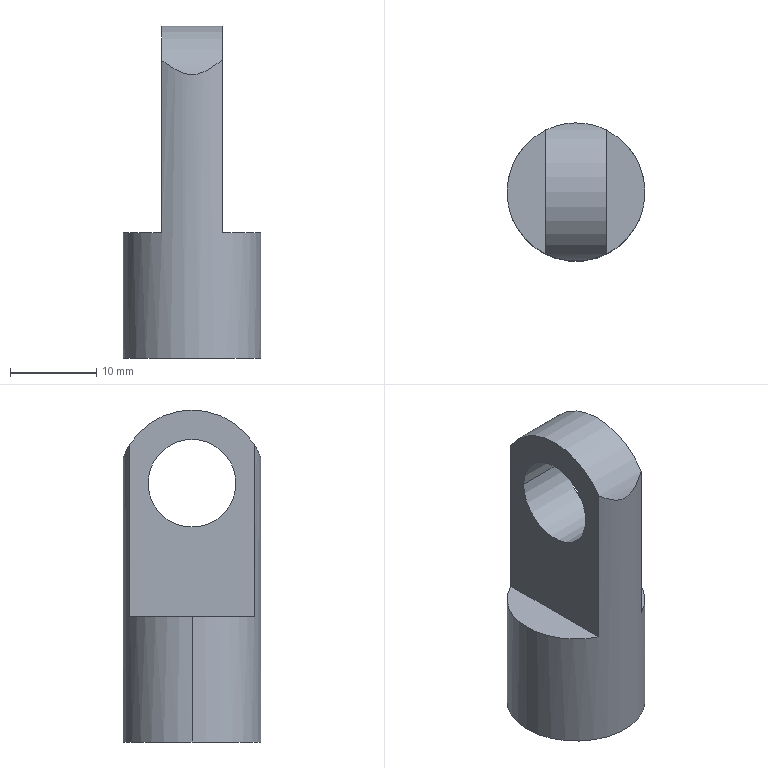Part | SolidWorks | features ICE 3, Extrusion 1, HoleWzd 1 | 1 solid | 14 faces | box 16 x 16 x 38.5 mm | volume 4330 mm3 | cylinder 7 | plane 5 | cone 2 | commonest cylinder face diameters 6.8 x2 10.2 x2 16 x2 17 x1
STEP:
#1=CARTESIAN_POINT('',(3.4,0.,12.));
#2=VERTEX_POINT('',#1);
#3=CARTESIAN_POINT('',(-3.4,0.,12.));
#4=VERTEX_POINT('',#3);
#5=CARTESIAN_POINT('',(0.,0.,12.));
#6=DIRECTION('',(0.,0.,-1.));
#7=DIRECTION('',(-1.,0.,0.));
#8=AXIS2_PLACEMENT_3D('',#5,#6,#7);
#9=CIRCLE('',#8,3.4);
#10=EDGE_CURVE('',#2,#4,#9,.T.);
#11=ORIENTED_EDGE('',*,*,#10,.F.);
#12=CARTESIAN_POINT('',(3.4,0.,0.));
#13=VERTEX_POINT('',#12);
#14=CARTESIAN_POINT('',(3.4,0.,0.));
#15=DIRECTION('',(0.,0.,-1.));
#16=VECTOR('',#15,1000.);
#17=LINE('',#14,#16);
#18=EDGE_CURVE('',#2,#13,#17,.T.);
#19=ORIENTED_EDGE('',*,*,#18,.T.);
#20=CARTESIAN_POINT('',(-3.4,0.,0.));
#21=VERTEX_POINT('',#20);
#22=CARTESIAN_POINT('',(0.,0.,0.));
#23=DIRECTION('',(0.,0.,-1.));
#24=DIRECTION('',(-1.,0.,0.));
#25=AXIS2_PLACEMENT_3D('',#22,#23,#24);
#26=CIRCLE('',#25,3.4);
#27=EDGE_CURVE('',#13,#21,#26,.T.);
#28=ORIENTED_EDGE('',*,*,#27,.T.);
#29=CARTESIAN_POINT('',(-3.4,0.,0.));
#30=DIRECTION('',(0.,0.,-1.));
#31=VECTOR('',#30,1000.);
#32=LINE('',#29,#31);
#33=EDGE_CURVE('',#4,#21,#32,.T.);
#34=ORIENTED_EDGE('',*,*,#33,.F.);
#35=EDGE_LOOP('',(#11,#19,#28,#34));
#36=FACE_OUTER_BOUND('',#35,.T.);
#37=CARTESIAN_POINT('',(0.,0.,0.));
#38=DIRECTION('',(0.,0.,-1.));
#39=DIRECTION('',(-1.,0.,0.));
#40=AXIS2_PLACEMENT_3D('',#37,#38,#39);
#41=CYLINDRICAL_SURFACE('',#40,3.4);
#42=ADVANCED_FACE('',(#36),#41,.F.);
#43=CARTESIAN_POINT('',(0.,0.,14.043));
#44=VERTEX_POINT('',#43);
#45=CARTESIAN_POINT('',(-3.4,0.,12.));
#46=DIRECTION('',(-0.8572,0.,-0.515));
#47=VECTOR('',#46,1000.);
#48=LINE('',#45,#47);
#49=EDGE_CURVE('',#44,#4,#48,.T.);
#50=ORIENTED_EDGE('',*,*,#49,.F.);
#51=CARTESIAN_POINT('',(3.4,0.,12.));
#52=DIRECTION('',(0.8572,0.,-0.515));
#53=VECTOR('',#52,1000.);
#54=LINE('',#51,#53);
#55=EDGE_CURVE('',#44,#2,#54,.T.);
#56=ORIENTED_EDGE('',*,*,#55,.T.);
#57=ORIENTED_EDGE('',*,*,#10,.T.);
#58=EDGE_LOOP('',(#50,#56,#57));
#59=FACE_OUTER_BOUND('',#58,.T.);
#60=CARTESIAN_POINT('',(0.,0.,12.));
#61=DIRECTION('',(0.,0.,-1.));
#62=DIRECTION('',(-1.,0.,0.));
#63=AXIS2_PLACEMENT_3D('',#60,#61,#62);
#64=CONICAL_SURFACE('',#63,3.4,1.03);
#65=ADVANCED_FACE('',(#59),#64,.F.);
#66=CARTESIAN_POINT('',(-3.5,-5.1,30.));
#67=VERTEX_POINT('',#66);
#68=CARTESIAN_POINT('',(-3.5,5.1,30.));
#69=VERTEX_POINT('',#68);
#70=CARTESIAN_POINT('',(-3.5,0.,30.));
#71=DIRECTION('',(1.,0.,0.));
#72=DIRECTION('',(0.,0.,-1.));
#73=AXIS2_PLACEMENT_3D('',#70,#71,#72);
#74=CIRCLE('',#73,5.1);
#75=EDGE_CURVE('',#67,#69,#74,.T.);
#76=ORIENTED_EDGE('',*,*,#75,.F.);
#77=CARTESIAN_POINT('',(3.5,-5.1,30.));
#78=VERTEX_POINT('',#77);
#79=CARTESIAN_POINT('',(-20.5,-5.1,30.));
#80=DIRECTION('',(1.,0.,0.));
#81=VECTOR('',#80,1000.);
#82=LINE('',#79,#81);
#83=EDGE_CURVE('',#67,#78,#82,.T.);
#84=ORIENTED_EDGE('',*,*,#83,.T.);
#85=CARTESIAN_POINT('',(3.5,5.1,30.));
#86=VERTEX_POINT('',#85);
#87=CARTESIAN_POINT('',(3.5,0.,30.));
#88=DIRECTION('',(1.,0.,0.));
#89=DIRECTION('',(0.,1.,0.));
#90=AXIS2_PLACEMENT_3D('',#87,#88,#89);
#91=CIRCLE('',#90,5.1);
#92=EDGE_CURVE('',#78,#86,#91,.T.);
#93=ORIENTED_EDGE('',*,*,#92,.T.);
#94=CARTESIAN_POINT('',(-20.5,5.1,30.));
#95=DIRECTION('',(1.,0.,0.));
#96=VECTOR('',#95,1000.);
#97=LINE('',#94,#96);
#98=EDGE_CURVE('',#69,#86,#97,.T.);
#99=ORIENTED_EDGE('',*,*,#98,.F.);
#100=EDGE_LOOP('',(#76,#84,#93,#99));
#101=FACE_OUTER_BOUND('',#100,.T.);
#102=CARTESIAN_POINT('',(-20.5,0.,30.));
#103=DIRECTION('',(1.,0.,0.));
#104=DIRECTION('',(0.,1.,0.));
#105=AXIS2_PLACEMENT_3D('',#102,#103,#104);
#106=CYLINDRICAL_SURFACE('',#105,5.1);
#107=ADVANCED_FACE('',(#101),#106,.F.);
#108=CARTESIAN_POINT('',(8.,0.,14.5));
#109=VERTEX_POINT('',#108);
#110=CARTESIAN_POINT('',(3.5,7.194,14.5));
#111=VERTEX_POINT('',#110);
#112=CARTESIAN_POINT('',(0.,0.,14.5));
#113=DIRECTION('',(0.,0.,1.));
#114=DIRECTION('',(1.,0.,0.));
#115=AXIS2_PLACEMENT_3D('',#112,#113,#114);
#116=CIRCLE('',#115,8.);
#117=EDGE_CURVE('',#109,#111,#116,.T.);
#118=ORIENTED_EDGE('',*,*,#117,.F.);
#119=CARTESIAN_POINT('',(8.,0.,0.));
#120=VERTEX_POINT('',#119);
#121=CARTESIAN_POINT('',(8.,0.,38.5));
#122=DIRECTION('',(0.,0.,-1.));
#123=VECTOR('',#122,1000.);
#124=LINE('',#121,#123);
#125=EDGE_CURVE('',#109,#120,#124,.T.);
#126=ORIENTED_EDGE('',*,*,#125,.T.);
#127=CARTESIAN_POINT('',(-8.,0.,0.));
#128=VERTEX_POINT('',#127);
#129=CARTESIAN_POINT('',(0.,0.,0.));
#130=DIRECTION('',(0.,0.,1.));
#131=DIRECTION('',(1.,0.,0.));
#132=AXIS2_PLACEMENT_3D('',#129,#130,#131);
#133=CIRCLE('',#132,8.);
#134=EDGE_CURVE('',#120,#128,#133,.T.);
#135=ORIENTED_EDGE('',*,*,#134,.T.);
#136=CARTESIAN_POINT('',(-8.,0.,14.5));
#137=VERTEX_POINT('',#136);
#138=CARTESIAN_POINT('',(-8.,0.,38.5));
#139=DIRECTION('',(0.,0.,-1.));
#140=VECTOR('',#139,1000.);
#141=LINE('',#138,#140);
#142=EDGE_CURVE('',#137,#128,#141,.T.);
#143=ORIENTED_EDGE('',*,*,#142,.F.);
#144=CARTESIAN_POINT('',(-3.5,7.194,14.5));
#145=VERTEX_POINT('',#144);
#146=CARTESIAN_POINT('',(0.,0.,14.5));
#147=DIRECTION('',(0.,0.,1.));
#148=DIRECTION('',(1.,0.,0.));
#149=AXIS2_PLACEMENT_3D('',#146,#147,#148);
#150=CIRCLE('',#149,8.);
#151=EDGE_CURVE('',#145,#137,#150,.T.);
#152=ORIENTED_EDGE('',*,*,#151,.F.);
#153=CARTESIAN_POINT('',(-3.5,7.194,34.528));
#154=VERTEX_POINT('',#153);
#155=CARTESIAN_POINT('',(-3.5,7.194,38.5));
#156=DIRECTION('',(0.,0.,1.));
#157=VECTOR('',#156,1000.);
#158=LINE('',#155,#157);
#159=EDGE_CURVE('',#145,#154,#158,.T.);
#160=ORIENTED_EDGE('',*,*,#159,.T.);
#161=CARTESIAN_POINT('',(3.5,7.194,34.528));
#162=VERTEX_POINT('',#161);
#163=CARTESIAN_POINT('',(-3.5,7.194,34.528));
#164=CARTESIAN_POINT('',(-3.254,7.314,34.337));
#165=CARTESIAN_POINT('',(-2.999,7.422,34.148));
#166=CARTESIAN_POINT('',(-2.468,7.615,33.782));
#167=CARTESIAN_POINT('',(-2.191,7.7,33.605));
#168=CARTESIAN_POINT('',(-1.758,7.806,33.365));
#169=CARTESIAN_POINT('',(-1.61,7.838,33.29));
#170=CARTESIAN_POINT('',(-1.307,7.894,33.153));
#171=CARTESIAN_POINT('',(-1.15,7.919,33.09));
#172=CARTESIAN_POINT('',(-0.8316,7.958,32.986));
#173=CARTESIAN_POINT('',(-0.6695,7.974,32.945));
#174=CARTESIAN_POINT('',(-0.3382,7.995,32.888));
#175=CARTESIAN_POINT('',(-0.167,8.,32.872));
#176=CARTESIAN_POINT('',(0.1699,8.,32.872));
#177=CARTESIAN_POINT('',(0.3366,7.995,32.887));
#178=CARTESIAN_POINT('',(0.6668,7.974,32.944));
#179=CARTESIAN_POINT('',(0.8317,7.958,32.986));
#180=CARTESIAN_POINT('',(1.31,7.899,33.143));
#181=CARTESIAN_POINT('',(1.609,7.842,33.284));
#182=CARTESIAN_POINT('',(2.186,7.701,33.602));
#183=CARTESIAN_POINT('',(2.463,7.617,33.779));
#184=CARTESIAN_POINT('',(2.994,7.424,34.145));
#185=CARTESIAN_POINT('',(3.251,7.315,34.335));
#186=CARTESIAN_POINT('',(3.5,7.194,34.528));
#187=B_SPLINE_CURVE_WITH_KNOTS('',3,(#163,#164,#165,#166,#167,#168,#169,#170,#171,#172,#173,#174,#175,#176,#177,#178,#179,#180,#181,#182,#183,#184,#185,#186),.UNSPECIFIED.,.F.,.F.,(4,2,2,2,2,2,2,2,2,2,2,4),(0.009914,0.01092,0.01192,0.01242,0.01292,0.01343,0.01393,0.01443,0.01493,0.01593,0.01694,0.01794),.UNSPECIFIED.);
#188=EDGE_CURVE('',#154,#162,#187,.T.);
#189=ORIENTED_EDGE('',*,*,#188,.T.);
#190=CARTESIAN_POINT('',(3.5,7.194,38.5));
#191=DIRECTION('',(0.,0.,-1.));
#192=VECTOR('',#191,1000.);
#193=LINE('',#190,#192);
#194=EDGE_CURVE('',#162,#111,#193,.T.);
#195=ORIENTED_EDGE('',*,*,#194,.T.);
#196=EDGE_LOOP('',(#118,#126,#135,#143,#152,#160,#189,#195));
#197=FACE_OUTER_BOUND('',#196,.T.);
#198=CARTESIAN_POINT('',(0.,0.,38.5));
#199=DIRECTION('',(0.,0.,-1.));
#200=DIRECTION('',(-1.,0.,0.));
#201=AXIS2_PLACEMENT_3D('',#198,#199,#200);
#202=CYLINDRICAL_SURFACE('',#201,8.);
#203=ADVANCED_FACE('',(#197),#202,.T.);
#204=CARTESIAN_POINT('',(-3.5,0.,30.));
#205=DIRECTION('',(1.,0.,0.));
#206=DIRECTION('',(0.,0.,-1.));
#207=AXIS2_PLACEMENT_3D('',#204,#205,#206);
#208=CIRCLE('',#207,5.1);
#209=EDGE_CURVE('',#69,#67,#208,.T.);
#210=ORIENTED_EDGE('',*,*,#209,.T.);
#211=ORIENTED_EDGE('',*,*,#75,.T.);
#212=EDGE_LOOP('',(#210,#211));
#213=FACE_BOUND('',#212,.T.);
#214=CARTESIAN_POINT('',(-3.5,-7.194,34.528));
#215=VERTEX_POINT('',#214);
#216=CARTESIAN_POINT('',(-3.5,-7.194,14.5));
#217=VERTEX_POINT('',#216);
#218=CARTESIAN_POINT('',(-3.5,-7.194,38.5));
#219=DIRECTION('',(0.,0.,-1.));
#220=VECTOR('',#219,1000.);
#221=LINE('',#218,#220);
#222=EDGE_CURVE('',#215,#217,#221,.T.);
#223=ORIENTED_EDGE('',*,*,#222,.F.);
#224=CARTESIAN_POINT('',(-3.5,0.,30.));
#225=DIRECTION('',(-1.,0.,0.));
#226=DIRECTION('',(0.,0.,-1.));
#227=AXIS2_PLACEMENT_3D('',#224,#225,#226);
#228=CIRCLE('',#227,8.5);
#229=EDGE_CURVE('',#215,#154,#228,.T.);
#230=ORIENTED_EDGE('',*,*,#229,.T.);
#231=ORIENTED_EDGE('',*,*,#159,.F.);
#232=CARTESIAN_POINT('',(-3.5,8.,14.5));
#233=DIRECTION('',(0.,1.,0.));
#234=VECTOR('',#233,1000.);
#235=LINE('',#232,#234);
#236=EDGE_CURVE('',#217,#145,#235,.T.);
#237=ORIENTED_EDGE('',*,*,#236,.F.);
#238=EDGE_LOOP('',(#223,#230,#231,#237));
#239=FACE_OUTER_BOUND('',#238,.T.);
#240=CARTESIAN_POINT('',(-3.5,8.,14.5));
#241=DIRECTION('',(1.,0.,0.));
#242=DIRECTION('',(0.,0.,-1.));
#243=AXIS2_PLACEMENT_3D('',#240,#241,#242);
#244=PLANE('',#243);
#245=ADVANCED_FACE('',(#213,#239),#244,.F.);
#246=CARTESIAN_POINT('',(3.5,0.,30.));
#247=DIRECTION('',(1.,0.,0.));
#248=DIRECTION('',(0.,1.,0.));
#249=AXIS2_PLACEMENT_3D('',#246,#247,#248);
#250=CIRCLE('',#249,5.1);
#251=EDGE_CURVE('',#86,#78,#250,.T.);
#252=ORIENTED_EDGE('',*,*,#251,.F.);
#253=ORIENTED_EDGE('',*,*,#92,.F.);
#254=EDGE_LOOP('',(#252,#253));
#255=FACE_BOUND('',#254,.T.);
#256=ORIENTED_EDGE('',*,*,#194,.F.);
#257=CARTESIAN_POINT('',(3.5,-7.194,34.528));
#258=VERTEX_POINT('',#257);
#259=CARTESIAN_POINT('',(3.5,0.,30.));
#260=DIRECTION('',(1.,0.,0.));
#261=DIRECTION('',(0.,-1.,0.));
#262=AXIS2_PLACEMENT_3D('',#259,#260,#261);
#263=CIRCLE('',#262,8.5);
#264=EDGE_CURVE('',#162,#258,#263,.T.);
#265=ORIENTED_EDGE('',*,*,#264,.T.);
#266=CARTESIAN_POINT('',(3.5,-7.194,14.5));
#267=VERTEX_POINT('',#266);
#268=CARTESIAN_POINT('',(3.5,-7.194,38.5));
#269=DIRECTION('',(0.,0.,1.));
#270=VECTOR('',#269,1000.);
#271=LINE('',#268,#270);
#272=EDGE_CURVE('',#267,#258,#271,.T.);
#273=ORIENTED_EDGE('',*,*,#272,.F.);
#274=CARTESIAN_POINT('',(3.5,8.,14.5));
#275=DIRECTION('',(0.,-1.,0.));
#276=VECTOR('',#275,1000.);
#277=LINE('',#274,#276);
#278=EDGE_CURVE('',#111,#267,#277,.T.);
#279=ORIENTED_EDGE('',*,*,#278,.F.);
#280=EDGE_LOOP('',(#256,#265,#273,#279));
#281=FACE_OUTER_BOUND('',#280,.T.);
#282=CARTESIAN_POINT('',(3.5,8.,14.5));
#283=DIRECTION('',(-1.,0.,0.));
#284=DIRECTION('',(0.,-1.,0.));
#285=AXIS2_PLACEMENT_3D('',#282,#283,#284);
#286=PLANE('',#285);
#287=ADVANCED_FACE('',(#255,#281),#286,.F.);
#288=ORIENTED_EDGE('',*,*,#125,.F.);
#289=CARTESIAN_POINT('',(0.,0.,14.5));
#290=DIRECTION('',(0.,0.,1.));
#291=DIRECTION('',(1.,0.,0.));
#292=AXIS2_PLACEMENT_3D('',#289,#290,#291);
#293=CIRCLE('',#292,8.);
#294=EDGE_CURVE('',#267,#109,#293,.T.);
#295=ORIENTED_EDGE('',*,*,#294,.F.);
#296=ORIENTED_EDGE('',*,*,#272,.T.);
#297=CARTESIAN_POINT('',(3.5,-7.194,34.528));
#298=CARTESIAN_POINT('',(3.25,-7.315,34.335));
#299=CARTESIAN_POINT('',(2.994,-7.424,34.145));
#300=CARTESIAN_POINT('',(2.463,-7.617,33.779));
#301=CARTESIAN_POINT('',(2.186,-7.701,33.602));
#302=CARTESIAN_POINT('',(1.609,-7.842,33.283));
#303=CARTESIAN_POINT('',(1.309,-7.899,33.142));
#304=CARTESIAN_POINT('',(0.8311,-7.958,32.986));
#305=CARTESIAN_POINT('',(0.666,-7.974,32.944));
#306=CARTESIAN_POINT('',(0.3347,-7.995,32.887));
#307=CARTESIAN_POINT('',(0.1674,-8.,32.872));
#308=CARTESIAN_POINT('',(-0.1706,-8.,32.872));
#309=CARTESIAN_POINT('',(-0.3414,-7.994,32.888));
#310=CARTESIAN_POINT('',(-0.6727,-7.973,32.945));
#311=CARTESIAN_POINT('',(-0.8351,-7.958,32.987));
#312=CARTESIAN_POINT('',(-1.155,-7.918,33.092));
#313=CARTESIAN_POINT('',(-1.311,-7.893,33.155));
#314=CARTESIAN_POINT('',(-1.613,-7.837,33.292));
#315=CARTESIAN_POINT('',(-1.76,-7.805,33.367));
#316=CARTESIAN_POINT('',(-2.191,-7.7,33.605));
#317=CARTESIAN_POINT('',(-2.466,-7.616,33.781));
#318=CARTESIAN_POINT('',(-2.999,-7.422,34.148));
#319=CARTESIAN_POINT('',(-3.253,-7.314,34.337));
#320=CARTESIAN_POINT('',(-3.5,-7.194,34.528));
#321=B_SPLINE_CURVE_WITH_KNOTS('',3,(#297,#298,#299,#300,#301,#302,#303,#304,#305,#306,#307,#308,#309,#310,#311,#312,#313,#314,#315,#316,#317,#318,#319,#320),.UNSPECIFIED.,.F.,.F.,(4,2,2,2,2,2,2,2,2,2,2,4),(0.,0.00101,0.00202,0.003031,0.003536,0.004041,0.004546,0.005051,0.005556,0.006061,0.007072,0.008082),.UNSPECIFIED.);
#322=EDGE_CURVE('',#258,#215,#321,.T.);
#323=ORIENTED_EDGE('',*,*,#322,.T.);
#324=ORIENTED_EDGE('',*,*,#222,.T.);
#325=CARTESIAN_POINT('',(0.,0.,14.5));
#326=DIRECTION('',(0.,0.,1.));
#327=DIRECTION('',(1.,0.,0.));
#328=AXIS2_PLACEMENT_3D('',#325,#326,#327);
#329=CIRCLE('',#328,8.);
#330=EDGE_CURVE('',#137,#217,#329,.T.);
#331=ORIENTED_EDGE('',*,*,#330,.F.);
#332=ORIENTED_EDGE('',*,*,#142,.T.);
#333=CARTESIAN_POINT('',(0.,0.,0.));
#334=DIRECTION('',(0.,0.,1.));
#335=DIRECTION('',(1.,0.,0.));
#336=AXIS2_PLACEMENT_3D('',#333,#334,#335);
#337=CIRCLE('',#336,8.);
#338=EDGE_CURVE('',#128,#120,#337,.T.);
#339=ORIENTED_EDGE('',*,*,#338,.T.);
#340=EDGE_LOOP('',(#288,#295,#296,#323,#324,#331,#332,#339));
#341=FACE_OUTER_BOUND('',#340,.T.);
#342=CARTESIAN_POINT('',(0.,0.,38.5));
#343=DIRECTION('',(0.,0.,-1.));
#344=DIRECTION('',(-1.,0.,0.));
#345=AXIS2_PLACEMENT_3D('',#342,#343,#344);
#346=CYLINDRICAL_SURFACE('',#345,8.);
#347=ADVANCED_FACE('',(#341),#346,.T.);
#348=CARTESIAN_POINT('',(0.,0.,0.));
#349=DIRECTION('',(0.,0.,-1.));
#350=DIRECTION('',(-1.,0.,0.));
#351=AXIS2_PLACEMENT_3D('',#348,#349,#350);
#352=CIRCLE('',#351,3.4);
#353=EDGE_CURVE('',#21,#13,#352,.T.);
#354=ORIENTED_EDGE('',*,*,#353,.F.);
#355=ORIENTED_EDGE('',*,*,#27,.F.);
#356=EDGE_LOOP('',(#354,#355));
#357=FACE_BOUND('',#356,.T.);
#358=ORIENTED_EDGE('',*,*,#338,.F.);
#359=ORIENTED_EDGE('',*,*,#134,.F.);
#360=EDGE_LOOP('',(#358,#359));
#361=FACE_OUTER_BOUND('',#360,.T.);
#362=CARTESIAN_POINT('',(0.,0.,0.));
#363=DIRECTION('',(0.,0.,1.));
#364=DIRECTION('',(1.,0.,0.));
#365=AXIS2_PLACEMENT_3D('',#362,#363,#364);
#366=PLANE('',#365);
#367=ADVANCED_FACE('',(#357,#361),#366,.F.);
#368=ORIENTED_EDGE('',*,*,#151,.T.);
#369=ORIENTED_EDGE('',*,*,#330,.T.);
#370=ORIENTED_EDGE('',*,*,#236,.T.);
#371=EDGE_LOOP('',(#368,#369,#370));
#372=FACE_OUTER_BOUND('',#371,.T.);
#373=CARTESIAN_POINT('',(0.,0.,14.5));
#374=DIRECTION('',(0.,0.,1.));
#375=DIRECTION('',(1.,0.,0.));
#376=AXIS2_PLACEMENT_3D('',#373,#374,#375);
#377=PLANE('',#376);
#378=ADVANCED_FACE('',(#372),#377,.T.);
#379=ORIENTED_EDGE('',*,*,#294,.T.);
#380=ORIENTED_EDGE('',*,*,#117,.T.);
#381=ORIENTED_EDGE('',*,*,#278,.T.);
#382=EDGE_LOOP('',(#379,#380,#381));
#383=FACE_OUTER_BOUND('',#382,.T.);
#384=CARTESIAN_POINT('',(0.,0.,14.5));
#385=DIRECTION('',(0.,0.,1.));
#386=DIRECTION('',(1.,0.,0.));
#387=AXIS2_PLACEMENT_3D('',#384,#385,#386);
#388=PLANE('',#387);
#389=ADVANCED_FACE('',(#383),#388,.T.);
#390=ORIENTED_EDGE('',*,*,#83,.F.);
#391=ORIENTED_EDGE('',*,*,#209,.F.);
#392=ORIENTED_EDGE('',*,*,#98,.T.);
#393=ORIENTED_EDGE('',*,*,#251,.T.);
#394=EDGE_LOOP('',(#390,#391,#392,#393));
#395=FACE_OUTER_BOUND('',#394,.T.);
#396=CARTESIAN_POINT('',(-20.5,0.,30.));
#397=DIRECTION('',(1.,0.,0.));
#398=DIRECTION('',(0.,1.,0.));
#399=AXIS2_PLACEMENT_3D('',#396,#397,#398);
#400=CYLINDRICAL_SURFACE('',#399,5.1);
#401=ADVANCED_FACE('',(#395),#400,.F.);
#402=ORIENTED_EDGE('',*,*,#264,.F.);
#403=ORIENTED_EDGE('',*,*,#188,.F.);
#404=ORIENTED_EDGE('',*,*,#229,.F.);
#405=ORIENTED_EDGE('',*,*,#322,.F.);
#406=EDGE_LOOP('',(#402,#403,#404,#405));
#407=FACE_OUTER_BOUND('',#406,.T.);
#408=CARTESIAN_POINT('',(-8.,0.,30.));
#409=DIRECTION('',(1.,0.,0.));
#410=DIRECTION('',(0.,1.,0.));
#411=AXIS2_PLACEMENT_3D('',#408,#409,#410);
#412=CYLINDRICAL_SURFACE('',#411,8.5);
#413=ADVANCED_FACE('',(#407),#412,.T.);
#414=ORIENTED_EDGE('',*,*,#55,.F.);
#415=ORIENTED_EDGE('',*,*,#49,.T.);
#416=CARTESIAN_POINT('',(0.,0.,12.));
#417=DIRECTION('',(0.,0.,-1.));
#418=DIRECTION('',(-1.,0.,0.));
#419=AXIS2_PLACEMENT_3D('',#416,#417,#418);
#420=CIRCLE('',#419,3.4);
#421=EDGE_CURVE('',#4,#2,#420,.T.);
#422=ORIENTED_EDGE('',*,*,#421,.T.);
#423=EDGE_LOOP('',(#414,#415,#422));
#424=FACE_OUTER_BOUND('',#423,.T.);
#425=CARTESIAN_POINT('',(0.,0.,12.));
#426=DIRECTION('',(0.,0.,-1.));
#427=DIRECTION('',(-1.,0.,0.));
#428=AXIS2_PLACEMENT_3D('',#425,#426,#427);
#429=CONICAL_SURFACE('',#428,3.4,1.03);
#430=ADVANCED_FACE('',(#424),#429,.F.);
#431=ORIENTED_EDGE('',*,*,#18,.F.);
#432=ORIENTED_EDGE('',*,*,#421,.F.);
#433=ORIENTED_EDGE('',*,*,#33,.T.);
#434=ORIENTED_EDGE('',*,*,#353,.T.);
#435=EDGE_LOOP('',(#431,#432,#433,#434));
#436=FACE_OUTER_BOUND('',#435,.T.);
#437=CARTESIAN_POINT('',(0.,0.,0.));
#438=DIRECTION('',(0.,0.,-1.));
#439=DIRECTION('',(-1.,0.,0.));
#440=AXIS2_PLACEMENT_3D('',#437,#438,#439);
#441=CYLINDRICAL_SURFACE('',#440,3.4);
#442=ADVANCED_FACE('',(#436),#441,.F.);
#443=CLOSED_SHELL('',(#42,#65,#107,#203,#245,#287,#347,#367,#378,#389,#401,#413,#430,#442));
#444=MANIFOLD_SOLID_BREP('',#443);
#445=CARTESIAN_POINT('',(0.,0.,0.));
#446=DIRECTION('',(0.,0.,1.));
#447=DIRECTION('',(1.,0.,0.));
#448=AXIS2_PLACEMENT_3D('',#445,#446,#447);
#449=(LENGTH_UNIT()NAMED_UNIT(*)SI_UNIT(.MILLI.,.METRE.));
#450=UNCERTAINTY_MEASURE_WITH_UNIT(LENGTH_MEASURE(0.00001),#449,'','');
#451=(NAMED_UNIT(*)PLANE_ANGLE_UNIT()SI_UNIT($,.RADIAN.));
#452=(NAMED_UNIT(*)SI_UNIT($,.STERADIAN.)SOLID_ANGLE_UNIT());
#453=(GEOMETRIC_REPRESENTATION_CONTEXT(3)GLOBAL_UNCERTAINTY_ASSIGNED_CONTEXT((#450))GLOBAL_UNIT_ASSIGNED_CONTEXT((#449,#451,#452))REPRESENTATION_CONTEXT('',''));
#454=ADVANCED_BREP_SHAPE_REPRESENTATION('',(#444,#448),#453);